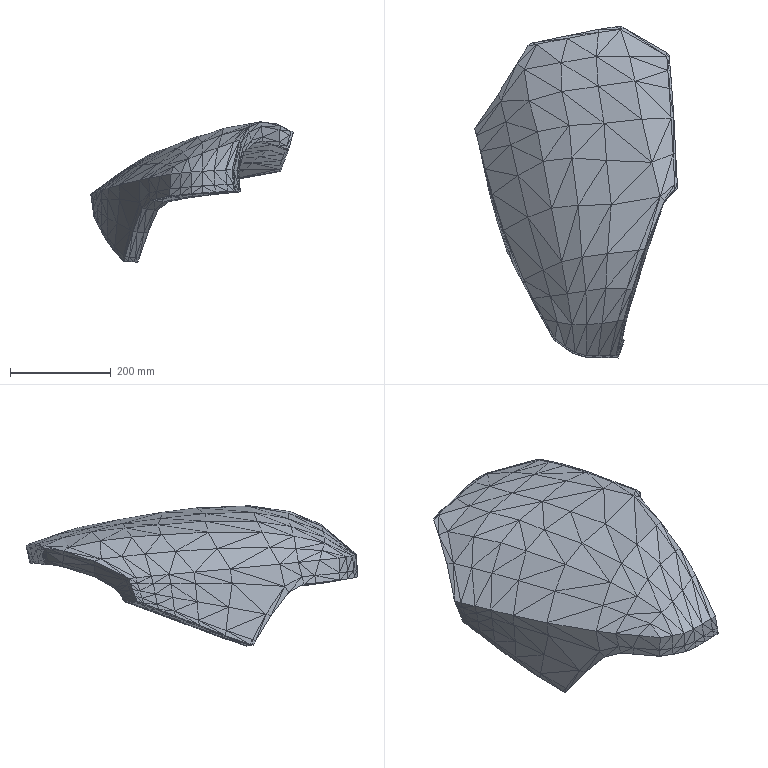Part | SolidWorks | features MirrorStock 1 | 1 solid | 769 faces | box 402.328 x 659.123 x 278.681 mm | volume 8547587 mm3 | plane 761 | cylinder 8 | commonest cylinder face diameters 12.5 x2 13 x2 32.5 x2 33 x2